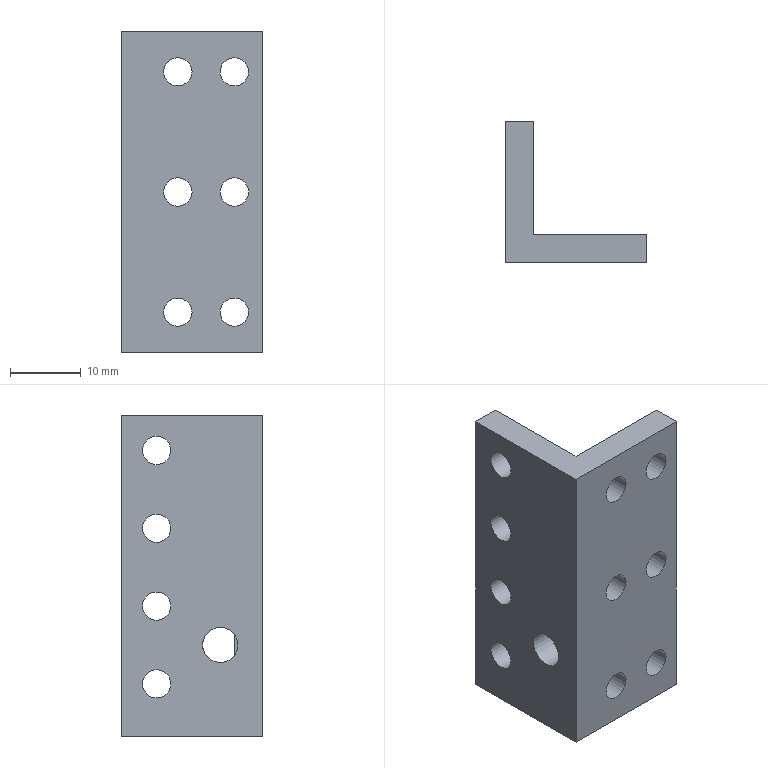Part | STEP file | 1-40.3 | 1 solid | 20 faces | box 20 x 20 x 45.5 mm | volume 5971 mm3 | cylinder 11 | plane 9 | commonest cylinder face diameters 4 x10 5 x1